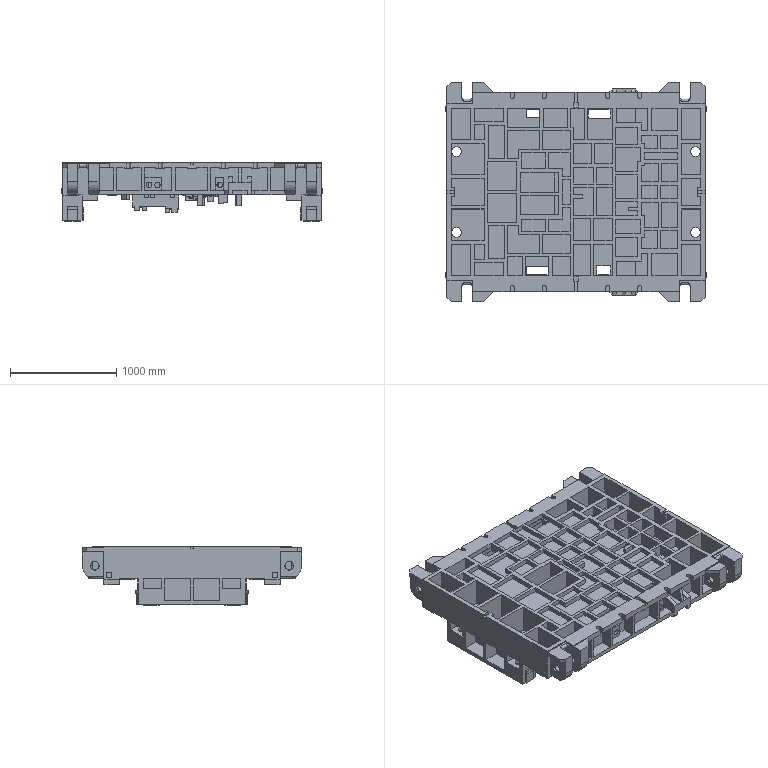Part | NX | features solid 2 | 1 solid | 2020 faces | box 2450 x 2070 x 555 mm | volume 626359236 mm3 | plane 1830 | cylinder 179 | torus 8 | spline 3 | commonest cylinder face diameters 83 x48 40 x28 30 x20 70 x16 79 x16 100 x10